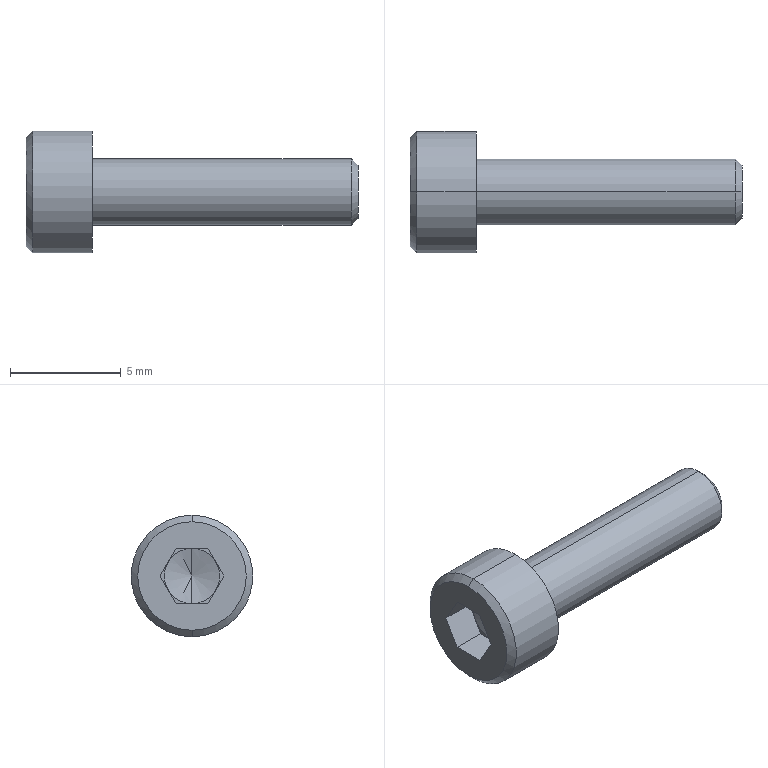Part | STEP file | 0246_303_SCB3-12 | 1 solid | 25 faces | box 15 x 5.5 x 5.5 mm | volume 146.269 mm3 | plane 15 | cone 6 | cylinder 4 | commonest cylinder face diameters 3 x2 5.5 x2